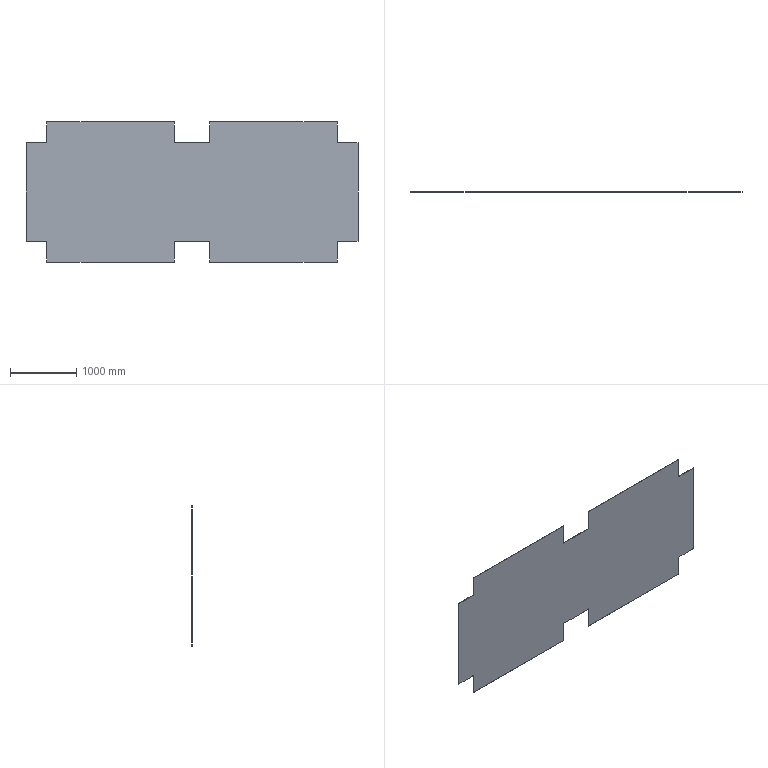Part | SolidWorks | features Extrusion 1 | 1 solid | 22 faces | box 5020 x 8 x 2120 mm | volume 79292800 mm3 | plane 22
STEP:
#1=CARTESIAN_POINT('',(-265.,0.,-1060.));
#2=VERTEX_POINT('',#1);
#3=CARTESIAN_POINT('',(-2195.,0.,-1060.));
#4=VERTEX_POINT('',#3);
#5=CARTESIAN_POINT('',(-265.,0.,-1060.));
#6=DIRECTION('',(-1.,0.,0.));
#7=VECTOR('',#6,1000.);
#8=LINE('',#5,#7);
#9=EDGE_CURVE('',#2,#4,#8,.T.);
#10=ORIENTED_EDGE('',*,*,#9,.T.);
#11=CARTESIAN_POINT('',(-2195.,8.,-1060.));
#12=VERTEX_POINT('',#11);
#13=CARTESIAN_POINT('',(-2195.,8.,-1060.));
#14=DIRECTION('',(0.,-1.,0.));
#15=VECTOR('',#14,1000.);
#16=LINE('',#13,#15);
#17=EDGE_CURVE('',#12,#4,#16,.T.);
#18=ORIENTED_EDGE('',*,*,#17,.F.);
#19=CARTESIAN_POINT('',(-265.,8.,-1060.));
#20=VERTEX_POINT('',#19);
#21=CARTESIAN_POINT('',(-265.,8.,-1060.));
#22=DIRECTION('',(-1.,0.,0.));
#23=VECTOR('',#22,1000.);
#24=LINE('',#21,#23);
#25=EDGE_CURVE('',#20,#12,#24,.T.);
#26=ORIENTED_EDGE('',*,*,#25,.F.);
#27=CARTESIAN_POINT('',(-265.,8.,-1060.));
#28=DIRECTION('',(0.,-1.,0.));
#29=VECTOR('',#28,1000.);
#30=LINE('',#27,#29);
#31=EDGE_CURVE('',#20,#2,#30,.T.);
#32=ORIENTED_EDGE('',*,*,#31,.T.);
#33=EDGE_LOOP('',(#10,#18,#26,#32));
#34=FACE_OUTER_BOUND('',#33,.T.);
#35=CARTESIAN_POINT('',(-265.,8.,-1060.));
#36=DIRECTION('',(0.,0.,1.));
#37=DIRECTION('',(1.,0.,0.));
#38=AXIS2_PLACEMENT_3D('',#35,#36,#37);
#39=PLANE('',#38);
#40=ADVANCED_FACE('',(#34),#39,.F.);
#41=CARTESIAN_POINT('',(-2195.,0.,-745.));
#42=VERTEX_POINT('',#41);
#43=CARTESIAN_POINT('',(-2195.,0.,-1060.));
#44=DIRECTION('',(0.,0.,1.));
#45=VECTOR('',#44,1000.);
#46=LINE('',#43,#45);
#47=EDGE_CURVE('',#4,#42,#46,.T.);
#48=ORIENTED_EDGE('',*,*,#47,.T.);
#49=CARTESIAN_POINT('',(-2195.,8.,-745.));
#50=VERTEX_POINT('',#49);
#51=CARTESIAN_POINT('',(-2195.,8.,-745.));
#52=DIRECTION('',(0.,-1.,0.));
#53=VECTOR('',#52,1000.);
#54=LINE('',#51,#53);
#55=EDGE_CURVE('',#50,#42,#54,.T.);
#56=ORIENTED_EDGE('',*,*,#55,.F.);
#57=CARTESIAN_POINT('',(-2195.,8.,-1060.));
#58=DIRECTION('',(0.,0.,1.));
#59=VECTOR('',#58,1000.);
#60=LINE('',#57,#59);
#61=EDGE_CURVE('',#12,#50,#60,.T.);
#62=ORIENTED_EDGE('',*,*,#61,.F.);
#63=ORIENTED_EDGE('',*,*,#17,.T.);
#64=EDGE_LOOP('',(#48,#56,#62,#63));
#65=FACE_OUTER_BOUND('',#64,.T.);
#66=CARTESIAN_POINT('',(-2195.,8.,-1060.));
#67=DIRECTION('',(1.,0.,0.));
#68=DIRECTION('',(0.,0.,-1.));
#69=AXIS2_PLACEMENT_3D('',#66,#67,#68);
#70=PLANE('',#69);
#71=ADVANCED_FACE('',(#65),#70,.F.);
#72=CARTESIAN_POINT('',(-2510.,0.,-745.));
#73=VERTEX_POINT('',#72);
#74=CARTESIAN_POINT('',(-2195.,0.,-745.));
#75=DIRECTION('',(-1.,0.,0.));
#76=VECTOR('',#75,1000.);
#77=LINE('',#74,#76);
#78=EDGE_CURVE('',#42,#73,#77,.T.);
#79=ORIENTED_EDGE('',*,*,#78,.T.);
#80=CARTESIAN_POINT('',(-2510.,8.,-745.));
#81=VERTEX_POINT('',#80);
#82=CARTESIAN_POINT('',(-2510.,8.,-745.));
#83=DIRECTION('',(0.,-1.,0.));
#84=VECTOR('',#83,1000.);
#85=LINE('',#82,#84);
#86=EDGE_CURVE('',#81,#73,#85,.T.);
#87=ORIENTED_EDGE('',*,*,#86,.F.);
#88=CARTESIAN_POINT('',(-2195.,8.,-745.));
#89=DIRECTION('',(-1.,0.,0.));
#90=VECTOR('',#89,1000.);
#91=LINE('',#88,#90);
#92=EDGE_CURVE('',#50,#81,#91,.T.);
#93=ORIENTED_EDGE('',*,*,#92,.F.);
#94=ORIENTED_EDGE('',*,*,#55,.T.);
#95=EDGE_LOOP('',(#79,#87,#93,#94));
#96=FACE_OUTER_BOUND('',#95,.T.);
#97=CARTESIAN_POINT('',(-2195.,8.,-745.));
#98=DIRECTION('',(0.,0.,1.));
#99=DIRECTION('',(1.,0.,0.));
#100=AXIS2_PLACEMENT_3D('',#97,#98,#99);
#101=PLANE('',#100);
#102=ADVANCED_FACE('',(#96),#101,.F.);
#103=CARTESIAN_POINT('',(-2510.,0.,745.));
#104=VERTEX_POINT('',#103);
#105=CARTESIAN_POINT('',(-2510.,0.,-745.));
#106=DIRECTION('',(0.,0.,1.));
#107=VECTOR('',#106,1000.);
#108=LINE('',#105,#107);
#109=EDGE_CURVE('',#73,#104,#108,.T.);
#110=ORIENTED_EDGE('',*,*,#109,.T.);
#111=CARTESIAN_POINT('',(-2510.,8.,745.));
#112=VERTEX_POINT('',#111);
#113=CARTESIAN_POINT('',(-2510.,8.,745.));
#114=DIRECTION('',(0.,-1.,0.));
#115=VECTOR('',#114,1000.);
#116=LINE('',#113,#115);
#117=EDGE_CURVE('',#112,#104,#116,.T.);
#118=ORIENTED_EDGE('',*,*,#117,.F.);
#119=CARTESIAN_POINT('',(-2510.,8.,-745.));
#120=DIRECTION('',(0.,0.,1.));
#121=VECTOR('',#120,1000.);
#122=LINE('',#119,#121);
#123=EDGE_CURVE('',#81,#112,#122,.T.);
#124=ORIENTED_EDGE('',*,*,#123,.F.);
#125=ORIENTED_EDGE('',*,*,#86,.T.);
#126=EDGE_LOOP('',(#110,#118,#124,#125));
#127=FACE_OUTER_BOUND('',#126,.T.);
#128=CARTESIAN_POINT('',(-2510.,8.,-745.));
#129=DIRECTION('',(1.,0.,0.));
#130=DIRECTION('',(0.,0.,-1.));
#131=AXIS2_PLACEMENT_3D('',#128,#129,#130);
#132=PLANE('',#131);
#133=ADVANCED_FACE('',(#127),#132,.F.);
#134=CARTESIAN_POINT('',(-2195.,0.,745.));
#135=VERTEX_POINT('',#134);
#136=CARTESIAN_POINT('',(-2195.,0.,745.));
#137=DIRECTION('',(1.,0.,0.));
#138=VECTOR('',#137,1000.);
#139=LINE('',#136,#138);
#140=EDGE_CURVE('',#104,#135,#139,.T.);
#141=ORIENTED_EDGE('',*,*,#140,.T.);
#142=CARTESIAN_POINT('',(-2195.,8.,745.));
#143=VERTEX_POINT('',#142);
#144=CARTESIAN_POINT('',(-2195.,8.,745.));
#145=DIRECTION('',(0.,-1.,0.));
#146=VECTOR('',#145,1000.);
#147=LINE('',#144,#146);
#148=EDGE_CURVE('',#143,#135,#147,.T.);
#149=ORIENTED_EDGE('',*,*,#148,.F.);
#150=CARTESIAN_POINT('',(-2195.,8.,745.));
#151=DIRECTION('',(1.,0.,0.));
#152=VECTOR('',#151,1000.);
#153=LINE('',#150,#152);
#154=EDGE_CURVE('',#112,#143,#153,.T.);
#155=ORIENTED_EDGE('',*,*,#154,.F.);
#156=ORIENTED_EDGE('',*,*,#117,.T.);
#157=EDGE_LOOP('',(#141,#149,#155,#156));
#158=FACE_OUTER_BOUND('',#157,.T.);
#159=CARTESIAN_POINT('',(-2195.,8.,745.));
#160=DIRECTION('',(0.,0.,-1.));
#161=DIRECTION('',(-1.,0.,0.));
#162=AXIS2_PLACEMENT_3D('',#159,#160,#161);
#163=PLANE('',#162);
#164=ADVANCED_FACE('',(#158),#163,.F.);
#165=CARTESIAN_POINT('',(-2195.,0.,1060.));
#166=VERTEX_POINT('',#165);
#167=CARTESIAN_POINT('',(-2195.,0.,1060.));
#168=DIRECTION('',(0.,0.,1.));
#169=VECTOR('',#168,1000.);
#170=LINE('',#167,#169);
#171=EDGE_CURVE('',#135,#166,#170,.T.);
#172=ORIENTED_EDGE('',*,*,#171,.T.);
#173=CARTESIAN_POINT('',(-2195.,8.,1060.));
#174=VERTEX_POINT('',#173);
#175=CARTESIAN_POINT('',(-2195.,8.,1060.));
#176=DIRECTION('',(0.,-1.,0.));
#177=VECTOR('',#176,1000.);
#178=LINE('',#175,#177);
#179=EDGE_CURVE('',#174,#166,#178,.T.);
#180=ORIENTED_EDGE('',*,*,#179,.F.);
#181=CARTESIAN_POINT('',(-2195.,8.,1060.));
#182=DIRECTION('',(0.,0.,1.));
#183=VECTOR('',#182,1000.);
#184=LINE('',#181,#183);
#185=EDGE_CURVE('',#143,#174,#184,.T.);
#186=ORIENTED_EDGE('',*,*,#185,.F.);
#187=ORIENTED_EDGE('',*,*,#148,.T.);
#188=EDGE_LOOP('',(#172,#180,#186,#187));
#189=FACE_OUTER_BOUND('',#188,.T.);
#190=CARTESIAN_POINT('',(-2195.,8.,1060.));
#191=DIRECTION('',(1.,0.,0.));
#192=DIRECTION('',(0.,0.,-1.));
#193=AXIS2_PLACEMENT_3D('',#190,#191,#192);
#194=PLANE('',#193);
#195=ADVANCED_FACE('',(#189),#194,.F.);
#196=CARTESIAN_POINT('',(-265.,0.,1060.));
#197=VERTEX_POINT('',#196);
#198=CARTESIAN_POINT('',(-265.,0.,1060.));
#199=DIRECTION('',(1.,0.,0.));
#200=VECTOR('',#199,1000.);
#201=LINE('',#198,#200);
#202=EDGE_CURVE('',#166,#197,#201,.T.);
#203=ORIENTED_EDGE('',*,*,#202,.T.);
#204=CARTESIAN_POINT('',(-265.,8.,1060.));
#205=VERTEX_POINT('',#204);
#206=CARTESIAN_POINT('',(-265.,8.,1060.));
#207=DIRECTION('',(0.,-1.,0.));
#208=VECTOR('',#207,1000.);
#209=LINE('',#206,#208);
#210=EDGE_CURVE('',#205,#197,#209,.T.);
#211=ORIENTED_EDGE('',*,*,#210,.F.);
#212=CARTESIAN_POINT('',(-265.,8.,1060.));
#213=DIRECTION('',(1.,0.,0.));
#214=VECTOR('',#213,1000.);
#215=LINE('',#212,#214);
#216=EDGE_CURVE('',#174,#205,#215,.T.);
#217=ORIENTED_EDGE('',*,*,#216,.F.);
#218=ORIENTED_EDGE('',*,*,#179,.T.);
#219=EDGE_LOOP('',(#203,#211,#217,#218));
#220=FACE_OUTER_BOUND('',#219,.T.);
#221=CARTESIAN_POINT('',(-265.,8.,1060.));
#222=DIRECTION('',(0.,0.,-1.));
#223=DIRECTION('',(-1.,0.,0.));
#224=AXIS2_PLACEMENT_3D('',#221,#222,#223);
#225=PLANE('',#224);
#226=ADVANCED_FACE('',(#220),#225,.F.);
#227=CARTESIAN_POINT('',(-265.,0.,745.));
#228=VERTEX_POINT('',#227);
#229=CARTESIAN_POINT('',(-265.,0.,1060.));
#230=DIRECTION('',(0.,0.,-1.));
#231=VECTOR('',#230,1000.);
#232=LINE('',#229,#231);
#233=EDGE_CURVE('',#197,#228,#232,.T.);
#234=ORIENTED_EDGE('',*,*,#233,.T.);
#235=CARTESIAN_POINT('',(-265.,8.,745.));
#236=VERTEX_POINT('',#235);
#237=CARTESIAN_POINT('',(-265.,8.,745.));
#238=DIRECTION('',(0.,-1.,0.));
#239=VECTOR('',#238,1000.);
#240=LINE('',#237,#239);
#241=EDGE_CURVE('',#236,#228,#240,.T.);
#242=ORIENTED_EDGE('',*,*,#241,.F.);
#243=CARTESIAN_POINT('',(-265.,8.,1060.));
#244=DIRECTION('',(0.,0.,-1.));
#245=VECTOR('',#244,1000.);
#246=LINE('',#243,#245);
#247=EDGE_CURVE('',#205,#236,#246,.T.);
#248=ORIENTED_EDGE('',*,*,#247,.F.);
#249=ORIENTED_EDGE('',*,*,#210,.T.);
#250=EDGE_LOOP('',(#234,#242,#248,#249));
#251=FACE_OUTER_BOUND('',#250,.T.);
#252=CARTESIAN_POINT('',(-265.,8.,1060.));
#253=DIRECTION('',(-1.,0.,0.));
#254=DIRECTION('',(0.,0.,1.));
#255=AXIS2_PLACEMENT_3D('',#252,#253,#254);
#256=PLANE('',#255);
#257=ADVANCED_FACE('',(#251),#256,.F.);
#258=CARTESIAN_POINT('',(265.,0.,745.));
#259=VERTEX_POINT('',#258);
#260=CARTESIAN_POINT('',(-265.,0.,745.));
#261=DIRECTION('',(1.,0.,0.));
#262=VECTOR('',#261,1000.);
#263=LINE('',#260,#262);
#264=EDGE_CURVE('',#228,#259,#263,.T.);
#265=ORIENTED_EDGE('',*,*,#264,.T.);
#266=CARTESIAN_POINT('',(265.,8.,745.));
#267=VERTEX_POINT('',#266);
#268=CARTESIAN_POINT('',(265.,8.,745.));
#269=DIRECTION('',(0.,-1.,0.));
#270=VECTOR('',#269,1000.);
#271=LINE('',#268,#270);
#272=EDGE_CURVE('',#267,#259,#271,.T.);
#273=ORIENTED_EDGE('',*,*,#272,.F.);
#274=CARTESIAN_POINT('',(-265.,8.,745.));
#275=DIRECTION('',(1.,0.,0.));
#276=VECTOR('',#275,1000.);
#277=LINE('',#274,#276);
#278=EDGE_CURVE('',#236,#267,#277,.T.);
#279=ORIENTED_EDGE('',*,*,#278,.F.);
#280=ORIENTED_EDGE('',*,*,#241,.T.);
#281=EDGE_LOOP('',(#265,#273,#279,#280));
#282=FACE_OUTER_BOUND('',#281,.T.);
#283=CARTESIAN_POINT('',(-265.,8.,745.));
#284=DIRECTION('',(0.,0.,-1.));
#285=DIRECTION('',(-1.,0.,0.));
#286=AXIS2_PLACEMENT_3D('',#283,#284,#285);
#287=PLANE('',#286);
#288=ADVANCED_FACE('',(#282),#287,.F.);
#289=CARTESIAN_POINT('',(265.,0.,1060.));
#290=VERTEX_POINT('',#289);
#291=CARTESIAN_POINT('',(265.,0.,1060.));
#292=DIRECTION('',(0.,0.,1.));
#293=VECTOR('',#292,1000.);
#294=LINE('',#291,#293);
#295=EDGE_CURVE('',#259,#290,#294,.T.);
#296=ORIENTED_EDGE('',*,*,#295,.T.);
#297=CARTESIAN_POINT('',(265.,8.,1060.));
#298=VERTEX_POINT('',#297);
#299=CARTESIAN_POINT('',(265.,8.,1060.));
#300=DIRECTION('',(0.,-1.,0.));
#301=VECTOR('',#300,1000.);
#302=LINE('',#299,#301);
#303=EDGE_CURVE('',#298,#290,#302,.T.);
#304=ORIENTED_EDGE('',*,*,#303,.F.);
#305=CARTESIAN_POINT('',(265.,8.,1060.));
#306=DIRECTION('',(0.,0.,1.));
#307=VECTOR('',#306,1000.);
#308=LINE('',#305,#307);
#309=EDGE_CURVE('',#267,#298,#308,.T.);
#310=ORIENTED_EDGE('',*,*,#309,.F.);
#311=ORIENTED_EDGE('',*,*,#272,.T.);
#312=EDGE_LOOP('',(#296,#304,#310,#311));
#313=FACE_OUTER_BOUND('',#312,.T.);
#314=CARTESIAN_POINT('',(265.,8.,1060.));
#315=DIRECTION('',(1.,0.,0.));
#316=DIRECTION('',(0.,0.,-1.));
#317=AXIS2_PLACEMENT_3D('',#314,#315,#316);
#318=PLANE('',#317);
#319=ADVANCED_FACE('',(#313),#318,.F.);
#320=CARTESIAN_POINT('',(2195.,0.,1060.));
#321=VERTEX_POINT('',#320);
#322=CARTESIAN_POINT('',(2195.,0.,1060.));
#323=DIRECTION('',(1.,0.,0.));
#324=VECTOR('',#323,1000.);
#325=LINE('',#322,#324);
#326=EDGE_CURVE('',#290,#321,#325,.T.);
#327=ORIENTED_EDGE('',*,*,#326,.T.);
#328=CARTESIAN_POINT('',(2195.,8.,1060.));
#329=VERTEX_POINT('',#328);
#330=CARTESIAN_POINT('',(2195.,8.,1060.));
#331=DIRECTION('',(0.,-1.,0.));
#332=VECTOR('',#331,1000.);
#333=LINE('',#330,#332);
#334=EDGE_CURVE('',#329,#321,#333,.T.);
#335=ORIENTED_EDGE('',*,*,#334,.F.);
#336=CARTESIAN_POINT('',(2195.,8.,1060.));
#337=DIRECTION('',(1.,0.,0.));
#338=VECTOR('',#337,1000.);
#339=LINE('',#336,#338);
#340=EDGE_CURVE('',#298,#329,#339,.T.);
#341=ORIENTED_EDGE('',*,*,#340,.F.);
#342=ORIENTED_EDGE('',*,*,#303,.T.);
#343=EDGE_LOOP('',(#327,#335,#341,#342));
#344=FACE_OUTER_BOUND('',#343,.T.);
#345=CARTESIAN_POINT('',(2195.,8.,1060.));
#346=DIRECTION('',(0.,0.,-1.));
#347=DIRECTION('',(-1.,0.,0.));
#348=AXIS2_PLACEMENT_3D('',#345,#346,#347);
#349=PLANE('',#348);
#350=ADVANCED_FACE('',(#344),#349,.F.);
#351=CARTESIAN_POINT('',(2195.,0.,745.));
#352=VERTEX_POINT('',#351);
#353=CARTESIAN_POINT('',(2195.,0.,1060.));
#354=DIRECTION('',(0.,0.,-1.));
#355=VECTOR('',#354,1000.);
#356=LINE('',#353,#355);
#357=EDGE_CURVE('',#321,#352,#356,.T.);
#358=ORIENTED_EDGE('',*,*,#357,.T.);
#359=CARTESIAN_POINT('',(2195.,8.,745.));
#360=VERTEX_POINT('',#359);
#361=CARTESIAN_POINT('',(2195.,8.,745.));
#362=DIRECTION('',(0.,-1.,0.));
#363=VECTOR('',#362,1000.);
#364=LINE('',#361,#363);
#365=EDGE_CURVE('',#360,#352,#364,.T.);
#366=ORIENTED_EDGE('',*,*,#365,.F.);
#367=CARTESIAN_POINT('',(2195.,8.,1060.));
#368=DIRECTION('',(0.,0.,-1.));
#369=VECTOR('',#368,1000.);
#370=LINE('',#367,#369);
#371=EDGE_CURVE('',#329,#360,#370,.T.);
#372=ORIENTED_EDGE('',*,*,#371,.F.);
#373=ORIENTED_EDGE('',*,*,#334,.T.);
#374=EDGE_LOOP('',(#358,#366,#372,#373));
#375=FACE_OUTER_BOUND('',#374,.T.);
#376=CARTESIAN_POINT('',(2195.,8.,1060.));
#377=DIRECTION('',(-1.,0.,0.));
#378=DIRECTION('',(0.,0.,1.));
#379=AXIS2_PLACEMENT_3D('',#376,#377,#378);
#380=PLANE('',#379);
#381=ADVANCED_FACE('',(#375),#380,.F.);
#382=CARTESIAN_POINT('',(2510.,0.,745.));
#383=VERTEX_POINT('',#382);
#384=CARTESIAN_POINT('',(2195.,0.,745.));
#385=DIRECTION('',(1.,0.,0.));
#386=VECTOR('',#385,1000.);
#387=LINE('',#384,#386);
#388=EDGE_CURVE('',#352,#383,#387,.T.);
#389=ORIENTED_EDGE('',*,*,#388,.T.);
#390=CARTESIAN_POINT('',(2510.,8.,745.));
#391=VERTEX_POINT('',#390);
#392=CARTESIAN_POINT('',(2510.,8.,745.));
#393=DIRECTION('',(0.,-1.,0.));
#394=VECTOR('',#393,1000.);
#395=LINE('',#392,#394);
#396=EDGE_CURVE('',#391,#383,#395,.T.);
#397=ORIENTED_EDGE('',*,*,#396,.F.);
#398=CARTESIAN_POINT('',(2195.,8.,745.));
#399=DIRECTION('',(1.,0.,0.));
#400=VECTOR('',#399,1000.);
#401=LINE('',#398,#400);
#402=EDGE_CURVE('',#360,#391,#401,.T.);
#403=ORIENTED_EDGE('',*,*,#402,.F.);
#404=ORIENTED_EDGE('',*,*,#365,.T.);
#405=EDGE_LOOP('',(#389,#397,#403,#404));
#406=FACE_OUTER_BOUND('',#405,.T.);
#407=CARTESIAN_POINT('',(2195.,8.,745.));
#408=DIRECTION('',(0.,0.,-1.));
#409=DIRECTION('',(-1.,0.,0.));
#410=AXIS2_PLACEMENT_3D('',#407,#408,#409);
#411=PLANE('',#410);
#412=ADVANCED_FACE('',(#406),#411,.F.);
#413=CARTESIAN_POINT('',(2510.,0.,-745.));
#414=VERTEX_POINT('',#413);
#415=CARTESIAN_POINT('',(2510.,0.,-745.));
#416=DIRECTION('',(0.,0.,-1.));
#417=VECTOR('',#416,1000.);
#418=LINE('',#415,#417);
#419=EDGE_CURVE('',#383,#414,#418,.T.);
#420=ORIENTED_EDGE('',*,*,#419,.T.);
#421=CARTESIAN_POINT('',(2510.,8.,-745.));
#422=VERTEX_POINT('',#421);
#423=CARTESIAN_POINT('',(2510.,8.,-745.));
#424=DIRECTION('',(0.,-1.,0.));
#425=VECTOR('',#424,1000.);
#426=LINE('',#423,#425);
#427=EDGE_CURVE('',#422,#414,#426,.T.);
#428=ORIENTED_EDGE('',*,*,#427,.F.);
#429=CARTESIAN_POINT('',(2510.,8.,-745.));
#430=DIRECTION('',(0.,0.,-1.));
#431=VECTOR('',#430,1000.);
#432=LINE('',#429,#431);
#433=EDGE_CURVE('',#391,#422,#432,.T.);
#434=ORIENTED_EDGE('',*,*,#433,.F.);
#435=ORIENTED_EDGE('',*,*,#396,.T.);
#436=EDGE_LOOP('',(#420,#428,#434,#435));
#437=FACE_OUTER_BOUND('',#436,.T.);
#438=CARTESIAN_POINT('',(2510.,8.,-745.));
#439=DIRECTION('',(-1.,0.,0.));
#440=DIRECTION('',(0.,0.,1.));
#441=AXIS2_PLACEMENT_3D('',#438,#439,#440);
#442=PLANE('',#441);
#443=ADVANCED_FACE('',(#437),#442,.F.);
#444=CARTESIAN_POINT('',(2195.,0.,-745.));
#445=VERTEX_POINT('',#444);
#446=CARTESIAN_POINT('',(2195.,0.,-745.));
#447=DIRECTION('',(-1.,0.,0.));
#448=VECTOR('',#447,1000.);
#449=LINE('',#446,#448);
#450=EDGE_CURVE('',#414,#445,#449,.T.);
#451=ORIENTED_EDGE('',*,*,#450,.T.);
#452=CARTESIAN_POINT('',(2195.,8.,-745.));
#453=VERTEX_POINT('',#452);
#454=CARTESIAN_POINT('',(2195.,8.,-745.));
#455=DIRECTION('',(0.,-1.,0.));
#456=VECTOR('',#455,1000.);
#457=LINE('',#454,#456);
#458=EDGE_CURVE('',#453,#445,#457,.T.);
#459=ORIENTED_EDGE('',*,*,#458,.F.);
#460=CARTESIAN_POINT('',(2195.,8.,-745.));
#461=DIRECTION('',(-1.,0.,0.));
#462=VECTOR('',#461,1000.);
#463=LINE('',#460,#462);
#464=EDGE_CURVE('',#422,#453,#463,.T.);
#465=ORIENTED_EDGE('',*,*,#464,.F.);
#466=ORIENTED_EDGE('',*,*,#427,.T.);
#467=EDGE_LOOP('',(#451,#459,#465,#466));
#468=FACE_OUTER_BOUND('',#467,.T.);
#469=CARTESIAN_POINT('',(2195.,8.,-745.));
#470=DIRECTION('',(0.,0.,1.));
#471=DIRECTION('',(1.,0.,0.));
#472=AXIS2_PLACEMENT_3D('',#469,#470,#471);
#473=PLANE('',#472);
#474=ADVANCED_FACE('',(#468),#473,.F.);
#475=CARTESIAN_POINT('',(2195.,0.,-1060.));
#476=VERTEX_POINT('',#475);
#477=CARTESIAN_POINT('',(2195.,0.,-1060.));
#478=DIRECTION('',(0.,0.,-1.));
#479=VECTOR('',#478,1000.);
#480=LINE('',#477,#479);
#481=EDGE_CURVE('',#445,#476,#480,.T.);
#482=ORIENTED_EDGE('',*,*,#481,.T.);
#483=CARTESIAN_POINT('',(2195.,8.,-1060.));
#484=VERTEX_POINT('',#483);
#485=CARTESIAN_POINT('',(2195.,8.,-1060.));
#486=DIRECTION('',(0.,-1.,0.));
#487=VECTOR('',#486,1000.);
#488=LINE('',#485,#487);
#489=EDGE_CURVE('',#484,#476,#488,.T.);
#490=ORIENTED_EDGE('',*,*,#489,.F.);
#491=CARTESIAN_POINT('',(2195.,8.,-1060.));
#492=DIRECTION('',(0.,0.,-1.));
#493=VECTOR('',#492,1000.);
#494=LINE('',#491,#493);
#495=EDGE_CURVE('',#453,#484,#494,.T.);
#496=ORIENTED_EDGE('',*,*,#495,.F.);
#497=ORIENTED_EDGE('',*,*,#458,.T.);
#498=EDGE_LOOP('',(#482,#490,#496,#497));
#499=FACE_OUTER_BOUND('',#498,.T.);
#500=CARTESIAN_POINT('',(2195.,8.,-1060.));
#501=DIRECTION('',(-1.,0.,0.));
#502=DIRECTION('',(0.,0.,1.));
#503=AXIS2_PLACEMENT_3D('',#500,#501,#502);
#504=PLANE('',#503);
#505=ADVANCED_FACE('',(#499),#504,.F.);
#506=CARTESIAN_POINT('',(265.,0.,-1060.));
#507=VERTEX_POINT('',#506);
#508=CARTESIAN_POINT('',(2195.,0.,-1060.));
#509=DIRECTION('',(-1.,0.,0.));
#510=VECTOR('',#509,1000.);
#511=LINE('',#508,#510);
#512=EDGE_CURVE('',#476,#507,#511,.T.);
#513=ORIENTED_EDGE('',*,*,#512,.T.);
#514=CARTESIAN_POINT('',(265.,8.,-1060.));
#515=VERTEX_POINT('',#514);
#516=CARTESIAN_POINT('',(265.,8.,-1060.));
#517=DIRECTION('',(0.,-1.,0.));
#518=VECTOR('',#517,1000.);
#519=LINE('',#516,#518);
#520=EDGE_CURVE('',#515,#507,#519,.T.);
#521=ORIENTED_EDGE('',*,*,#520,.F.);
#522=CARTESIAN_POINT('',(2195.,8.,-1060.));
#523=DIRECTION('',(-1.,0.,0.));
#524=VECTOR('',#523,1000.);
#525=LINE('',#522,#524);
#526=EDGE_CURVE('',#484,#515,#525,.T.);
#527=ORIENTED_EDGE('',*,*,#526,.F.);
#528=ORIENTED_EDGE('',*,*,#489,.T.);
#529=EDGE_LOOP('',(#513,#521,#527,#528));
#530=FACE_OUTER_BOUND('',#529,.T.);
#531=CARTESIAN_POINT('',(2195.,8.,-1060.));
#532=DIRECTION('',(0.,0.,1.));
#533=DIRECTION('',(1.,0.,0.));
#534=AXIS2_PLACEMENT_3D('',#531,#532,#533);
#535=PLANE('',#534);
#536=ADVANCED_FACE('',(#530),#535,.F.);
#537=CARTESIAN_POINT('',(265.,0.,-745.));
#538=VERTEX_POINT('',#537);
#539=CARTESIAN_POINT('',(265.,0.,-1060.));
#540=DIRECTION('',(0.,0.,1.));
#541=VECTOR('',#540,1000.);
#542=LINE('',#539,#541);
#543=EDGE_CURVE('',#507,#538,#542,.T.);
#544=ORIENTED_EDGE('',*,*,#543,.T.);
#545=CARTESIAN_POINT('',(265.,8.,-745.));
#546=VERTEX_POINT('',#545);
#547=CARTESIAN_POINT('',(265.,8.,-745.));
#548=DIRECTION('',(0.,-1.,0.));
#549=VECTOR('',#548,1000.);
#550=LINE('',#547,#549);
#551=EDGE_CURVE('',#546,#538,#550,.T.);
#552=ORIENTED_EDGE('',*,*,#551,.F.);
#553=CARTESIAN_POINT('',(265.,8.,-1060.));
#554=DIRECTION('',(0.,0.,1.));
#555=VECTOR('',#554,1000.);
#556=LINE('',#553,#555);
#557=EDGE_CURVE('',#515,#546,#556,.T.);
#558=ORIENTED_EDGE('',*,*,#557,.F.);
#559=ORIENTED_EDGE('',*,*,#520,.T.);
#560=EDGE_LOOP('',(#544,#552,#558,#559));
#561=FACE_OUTER_BOUND('',#560,.T.);
#562=CARTESIAN_POINT('',(265.,8.,-1060.));
#563=DIRECTION('',(1.,0.,0.));
#564=DIRECTION('',(0.,0.,-1.));
#565=AXIS2_PLACEMENT_3D('',#562,#563,#564);
#566=PLANE('',#565);
#567=ADVANCED_FACE('',(#561),#566,.F.);
#568=CARTESIAN_POINT('',(-265.,0.,-745.));
#569=VERTEX_POINT('',#568);
#570=CARTESIAN_POINT('',(-265.,0.,-745.));
#571=DIRECTION('',(-1.,0.,0.));
#572=VECTOR('',#571,1000.);
#573=LINE('',#570,#572);
#574=EDGE_CURVE('',#538,#569,#573,.T.);
#575=ORIENTED_EDGE('',*,*,#574,.T.);
#576=CARTESIAN_POINT('',(-265.,8.,-745.));
#577=VERTEX_POINT('',#576);
#578=CARTESIAN_POINT('',(-265.,8.,-745.));
#579=DIRECTION('',(0.,-1.,0.));
#580=VECTOR('',#579,1000.);
#581=LINE('',#578,#580);
#582=EDGE_CURVE('',#577,#569,#581,.T.);
#583=ORIENTED_EDGE('',*,*,#582,.F.);
#584=CARTESIAN_POINT('',(-265.,8.,-745.));
#585=DIRECTION('',(-1.,0.,0.));
#586=VECTOR('',#585,1000.);
#587=LINE('',#584,#586);
#588=EDGE_CURVE('',#546,#577,#587,.T.);
#589=ORIENTED_EDGE('',*,*,#588,.F.);
#590=ORIENTED_EDGE('',*,*,#551,.T.);
#591=EDGE_LOOP('',(#575,#583,#589,#590));
#592=FACE_OUTER_BOUND('',#591,.T.);
#593=CARTESIAN_POINT('',(-265.,8.,-745.));
#594=DIRECTION('',(0.,0.,1.));
#595=DIRECTION('',(1.,0.,0.));
#596=AXIS2_PLACEMENT_3D('',#593,#594,#595);
#597=PLANE('',#596);
#598=ADVANCED_FACE('',(#592),#597,.F.);
#599=CARTESIAN_POINT('',(-265.,0.,-1060.));
#600=DIRECTION('',(0.,0.,-1.));
#601=VECTOR('',#600,1000.);
#602=LINE('',#599,#601);
#603=EDGE_CURVE('',#569,#2,#602,.T.);
#604=ORIENTED_EDGE('',*,*,#603,.T.);
#605=ORIENTED_EDGE('',*,*,#31,.F.);
#606=CARTESIAN_POINT('',(-265.,8.,-1060.));
#607=DIRECTION('',(0.,0.,-1.));
#608=VECTOR('',#607,1000.);
#609=LINE('',#606,#608);
#610=EDGE_CURVE('',#577,#20,#609,.T.);
#611=ORIENTED_EDGE('',*,*,#610,.F.);
#612=ORIENTED_EDGE('',*,*,#582,.T.);
#613=EDGE_LOOP('',(#604,#605,#611,#612));
#614=FACE_OUTER_BOUND('',#613,.T.);
#615=CARTESIAN_POINT('',(-265.,8.,-1060.));
#616=DIRECTION('',(-1.,0.,0.));
#617=DIRECTION('',(0.,0.,1.));
#618=AXIS2_PLACEMENT_3D('',#615,#616,#617);
#619=PLANE('',#618);
#620=ADVANCED_FACE('',(#614),#619,.F.);
#621=ORIENTED_EDGE('',*,*,#25,.T.);
#622=ORIENTED_EDGE('',*,*,#61,.T.);
#623=ORIENTED_EDGE('',*,*,#92,.T.);
#624=ORIENTED_EDGE('',*,*,#123,.T.);
#625=ORIENTED_EDGE('',*,*,#154,.T.);
#626=ORIENTED_EDGE('',*,*,#185,.T.);
#627=ORIENTED_EDGE('',*,*,#216,.T.);
#628=ORIENTED_EDGE('',*,*,#247,.T.);
#629=ORIENTED_EDGE('',*,*,#278,.T.);
#630=ORIENTED_EDGE('',*,*,#309,.T.);
#631=ORIENTED_EDGE('',*,*,#340,.T.);
#632=ORIENTED_EDGE('',*,*,#371,.T.);
#633=ORIENTED_EDGE('',*,*,#402,.T.);
#634=ORIENTED_EDGE('',*,*,#433,.T.);
#635=ORIENTED_EDGE('',*,*,#464,.T.);
#636=ORIENTED_EDGE('',*,*,#495,.T.);
#637=ORIENTED_EDGE('',*,*,#526,.T.);
#638=ORIENTED_EDGE('',*,*,#557,.T.);
#639=ORIENTED_EDGE('',*,*,#588,.T.);
#640=ORIENTED_EDGE('',*,*,#610,.T.);
#641=EDGE_LOOP('',(#621,#622,#623,#624,#625,#626,#627,#628,#629,#630,#631,#632,#633,#634,#635,#636,#637,#638,#639,#640));
#642=FACE_OUTER_BOUND('',#641,.T.);
#643=CARTESIAN_POINT('',(0.,8.,0.));
#644=DIRECTION('',(0.,1.,0.));
#645=DIRECTION('',(0.,0.,1.));
#646=AXIS2_PLACEMENT_3D('',#643,#644,#645);
#647=PLANE('',#646);
#648=ADVANCED_FACE('',(#642),#647,.T.);
#649=ORIENTED_EDGE('',*,*,#9,.F.);
#650=ORIENTED_EDGE('',*,*,#603,.F.);
#651=ORIENTED_EDGE('',*,*,#574,.F.);
#652=ORIENTED_EDGE('',*,*,#543,.F.);
#653=ORIENTED_EDGE('',*,*,#512,.F.);
#654=ORIENTED_EDGE('',*,*,#481,.F.);
#655=ORIENTED_EDGE('',*,*,#450,.F.);
#656=ORIENTED_EDGE('',*,*,#419,.F.);
#657=ORIENTED_EDGE('',*,*,#388,.F.);
#658=ORIENTED_EDGE('',*,*,#357,.F.);
#659=ORIENTED_EDGE('',*,*,#326,.F.);
#660=ORIENTED_EDGE('',*,*,#295,.F.);
#661=ORIENTED_EDGE('',*,*,#264,.F.);
#662=ORIENTED_EDGE('',*,*,#233,.F.);
#663=ORIENTED_EDGE('',*,*,#202,.F.);
#664=ORIENTED_EDGE('',*,*,#171,.F.);
#665=ORIENTED_EDGE('',*,*,#140,.F.);
#666=ORIENTED_EDGE('',*,*,#109,.F.);
#667=ORIENTED_EDGE('',*,*,#78,.F.);
#668=ORIENTED_EDGE('',*,*,#47,.F.);
#669=EDGE_LOOP('',(#649,#650,#651,#652,#653,#654,#655,#656,#657,#658,#659,#660,#661,#662,#663,#664,#665,#666,#667,#668));
#670=FACE_OUTER_BOUND('',#669,.T.);
#671=CARTESIAN_POINT('',(0.,0.,0.));
#672=DIRECTION('',(0.,1.,0.));
#673=DIRECTION('',(0.,0.,1.));
#674=AXIS2_PLACEMENT_3D('',#671,#672,#673);
#675=PLANE('',#674);
#676=ADVANCED_FACE('',(#670),#675,.F.);
#677=CLOSED_SHELL('',(#40,#71,#102,#133,#164,#195,#226,#257,#288,#319,#350,#381,#412,#443,#474,#505,#536,#567,#598,#620,#648,#676));
#678=MANIFOLD_SOLID_BREP('',#677);
#679=CARTESIAN_POINT('',(0.,0.,0.));
#680=DIRECTION('',(0.,0.,1.));
#681=DIRECTION('',(1.,0.,0.));
#682=AXIS2_PLACEMENT_3D('',#679,#680,#681);
#683=(LENGTH_UNIT()NAMED_UNIT(*)SI_UNIT(.MILLI.,.METRE.));
#684=UNCERTAINTY_MEASURE_WITH_UNIT(LENGTH_MEASURE(0.00001),#683,'','');
#685=(NAMED_UNIT(*)PLANE_ANGLE_UNIT()SI_UNIT($,.RADIAN.));
#686=(NAMED_UNIT(*)SI_UNIT($,.STERADIAN.)SOLID_ANGLE_UNIT());
#687=(GEOMETRIC_REPRESENTATION_CONTEXT(3)GLOBAL_UNCERTAINTY_ASSIGNED_CONTEXT((#684))GLOBAL_UNIT_ASSIGNED_CONTEXT((#683,#685,#686))REPRESENTATION_CONTEXT('',''));
#688=ADVANCED_BREP_SHAPE_REPRESENTATION('',(#678,#682),#687);